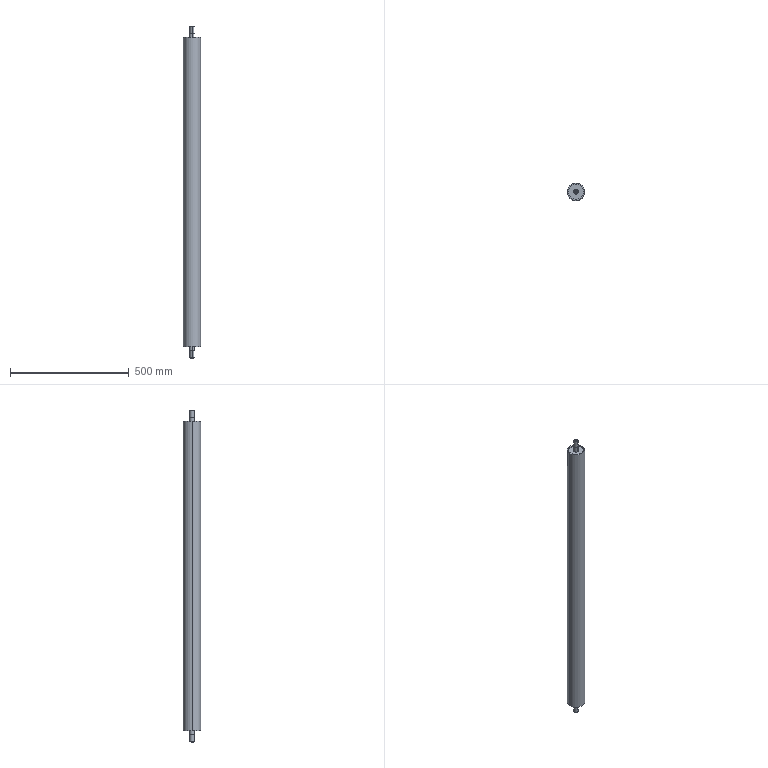Part | STEP file | Produce dryer-Driven part 2 | 1 solid | 44 faces | box 73 x 73 x 1397 mm | volume 1653987 mm3 | cylinder 22 | cone 12 | plane 10 | commonest cylinder face diameters 20 x6 64.52 x6 5 x4 17 x4 73 x2
STEP:
#1=CARTESIAN_POINT('',(2.5,0.,-683.5));
#2=VERTEX_POINT('',#1);
#3=CARTESIAN_POINT('',(-2.5,0.,-683.5));
#4=VERTEX_POINT('',#3);
#5=CARTESIAN_POINT('',(0.,0.,-683.5));
#6=DIRECTION('',(0.,0.,-1.));
#7=DIRECTION('',(-1.,0.,0.));
#8=AXIS2_PLACEMENT_3D('',#5,#6,#7);
#9=CIRCLE('',#8,2.5);
#10=EDGE_CURVE('',#2,#4,#9,.T.);
#11=ORIENTED_EDGE('',*,*,#10,.F.);
#12=CARTESIAN_POINT('',(2.5,0.,-698.5));
#13=VERTEX_POINT('',#12);
#14=CARTESIAN_POINT('',(2.5,0.,-698.5));
#15=DIRECTION('',(0.,0.,-1.));
#16=VECTOR('',#15,1000.);
#17=LINE('',#14,#16);
#18=EDGE_CURVE('',#2,#13,#17,.T.);
#19=ORIENTED_EDGE('',*,*,#18,.T.);
#20=CARTESIAN_POINT('',(-2.5,0.,-698.5));
#21=VERTEX_POINT('',#20);
#22=CARTESIAN_POINT('',(0.,0.,-698.5));
#23=DIRECTION('',(0.,0.,-1.));
#24=DIRECTION('',(-1.,0.,0.));
#25=AXIS2_PLACEMENT_3D('',#22,#23,#24);
#26=CIRCLE('',#25,2.5);
#27=EDGE_CURVE('',#13,#21,#26,.T.);
#28=ORIENTED_EDGE('',*,*,#27,.T.);
#29=CARTESIAN_POINT('',(-2.5,0.,-698.5));
#30=DIRECTION('',(0.,0.,-1.));
#31=VECTOR('',#30,1000.);
#32=LINE('',#29,#31);
#33=EDGE_CURVE('',#4,#21,#32,.T.);
#34=ORIENTED_EDGE('',*,*,#33,.F.);
#35=EDGE_LOOP('',(#11,#19,#28,#34));
#36=FACE_OUTER_BOUND('',#35,.T.);
#37=CARTESIAN_POINT('',(0.,0.,-698.5));
#38=DIRECTION('',(0.,0.,-1.));
#39=DIRECTION('',(-1.,0.,0.));
#40=AXIS2_PLACEMENT_3D('',#37,#38,#39);
#41=CYLINDRICAL_SURFACE('',#40,2.5);
#42=ADVANCED_FACE('',(#36),#41,.F.);
#43=CARTESIAN_POINT('',(0.,0.,-681.998));
#44=VERTEX_POINT('',#43);
#45=CARTESIAN_POINT('',(-2.5,0.,-683.5));
#46=DIRECTION('',(-0.8572,0.,-0.515));
#47=VECTOR('',#46,1000.);
#48=LINE('',#45,#47);
#49=EDGE_CURVE('',#44,#4,#48,.T.);
#50=ORIENTED_EDGE('',*,*,#49,.F.);
#51=CARTESIAN_POINT('',(2.5,0.,-683.5));
#52=DIRECTION('',(0.8572,0.,-0.515));
#53=VECTOR('',#52,1000.);
#54=LINE('',#51,#53);
#55=EDGE_CURVE('',#44,#2,#54,.T.);
#56=ORIENTED_EDGE('',*,*,#55,.T.);
#57=ORIENTED_EDGE('',*,*,#10,.T.);
#58=EDGE_LOOP('',(#50,#56,#57));
#59=FACE_OUTER_BOUND('',#58,.T.);
#60=CARTESIAN_POINT('',(0.,0.,-683.5));
#61=DIRECTION('',(0.,0.,-1.));
#62=DIRECTION('',(-1.,0.,0.));
#63=AXIS2_PLACEMENT_3D('',#60,#61,#62);
#64=CONICAL_SURFACE('',#63,2.5,1.03);
#65=ADVANCED_FACE('',(#59),#64,.F.);
#66=CARTESIAN_POINT('',(0.,-10.,-667.));
#67=VERTEX_POINT('',#66);
#68=CARTESIAN_POINT('',(0.,10.,-667.));
#69=VERTEX_POINT('',#68);
#70=CARTESIAN_POINT('',(0.,0.,-667.));
#71=DIRECTION('',(0.,0.,1.));
#72=DIRECTION('',(0.,-1.,0.));
#73=AXIS2_PLACEMENT_3D('',#70,#71,#72);
#74=CIRCLE('',#73,10.);
#75=EDGE_CURVE('',#67,#69,#74,.T.);
#76=ORIENTED_EDGE('',*,*,#75,.T.);
#77=CARTESIAN_POINT('',(0.,10.,-645.5));
#78=VERTEX_POINT('',#77);
#79=CARTESIAN_POINT('',(0.,10.,-698.5));
#80=DIRECTION('',(0.,0.,1.));
#81=VECTOR('',#80,1000.);
#82=LINE('',#79,#81);
#83=EDGE_CURVE('',#69,#78,#82,.T.);
#84=ORIENTED_EDGE('',*,*,#83,.T.);
#85=CARTESIAN_POINT('',(0.,-10.,-645.5));
#86=VERTEX_POINT('',#85);
#87=CARTESIAN_POINT('',(0.,0.,-645.5));
#88=DIRECTION('',(0.,0.,-1.));
#89=DIRECTION('',(-1.,0.,0.));
#90=AXIS2_PLACEMENT_3D('',#87,#88,#89);
#91=CIRCLE('',#90,10.);
#92=EDGE_CURVE('',#78,#86,#91,.T.);
#93=ORIENTED_EDGE('',*,*,#92,.T.);
#94=CARTESIAN_POINT('',(0.,-10.,-698.5));
#95=DIRECTION('',(0.,0.,1.));
#96=VECTOR('',#95,1000.);
#97=LINE('',#94,#96);
#98=EDGE_CURVE('',#67,#86,#97,.T.);
#99=ORIENTED_EDGE('',*,*,#98,.F.);
#100=EDGE_LOOP('',(#76,#84,#93,#99));
#101=FACE_OUTER_BOUND('',#100,.T.);
#102=CARTESIAN_POINT('',(0.,0.,-698.5));
#103=DIRECTION('',(0.,0.,1.));
#104=DIRECTION('',(0.,-1.,0.));
#105=AXIS2_PLACEMENT_3D('',#102,#103,#104);
#106=CYLINDRICAL_SURFACE('',#105,10.);
#107=ADVANCED_FACE('',(#101),#106,.T.);
#108=CARTESIAN_POINT('',(0.,9.5,-667.5));
#109=VERTEX_POINT('',#108);
#110=CARTESIAN_POINT('',(0.,-9.5,-667.5));
#111=VERTEX_POINT('',#110);
#112=CARTESIAN_POINT('',(0.,0.,-667.5));
#113=DIRECTION('',(0.,0.,-1.));
#114=DIRECTION('',(0.,-1.,0.));
#115=AXIS2_PLACEMENT_3D('',#112,#113,#114);
#116=CIRCLE('',#115,9.5);
#117=EDGE_CURVE('',#109,#111,#116,.T.);
#118=ORIENTED_EDGE('',*,*,#117,.F.);
#119=CARTESIAN_POINT('',(0.,10.,-667.));
#120=DIRECTION('',(0.,0.7071,0.7071));
#121=VECTOR('',#120,1000.);
#122=LINE('',#119,#121);
#123=EDGE_CURVE('',#109,#69,#122,.T.);
#124=ORIENTED_EDGE('',*,*,#123,.T.);
#125=ORIENTED_EDGE('',*,*,#75,.F.);
#126=CARTESIAN_POINT('',(0.,-10.,-667.));
#127=DIRECTION('',(0.,-0.7071,0.7071));
#128=VECTOR('',#127,1000.);
#129=LINE('',#126,#128);
#130=EDGE_CURVE('',#111,#67,#129,.T.);
#131=ORIENTED_EDGE('',*,*,#130,.F.);
#132=EDGE_LOOP('',(#118,#124,#125,#131));
#133=FACE_OUTER_BOUND('',#132,.T.);
#134=CARTESIAN_POINT('',(0.,0.,-667.));
#135=DIRECTION('',(0.,0.,1.));
#136=DIRECTION('',(0.,-1.,0.));
#137=AXIS2_PLACEMENT_3D('',#134,#135,#136);
#138=CONICAL_SURFACE('',#137,10.,0.7854);
#139=ADVANCED_FACE('',(#133),#138,.T.);
#140=CARTESIAN_POINT('',(0.,-8.5,-698.));
#141=VERTEX_POINT('',#140);
#142=CARTESIAN_POINT('',(0.,8.5,-698.));
#143=VERTEX_POINT('',#142);
#144=CARTESIAN_POINT('',(0.,0.,-698.));
#145=DIRECTION('',(0.,0.,1.));
#146=DIRECTION('',(0.,-1.,0.));
#147=AXIS2_PLACEMENT_3D('',#144,#145,#146);
#148=CIRCLE('',#147,8.5);
#149=EDGE_CURVE('',#141,#143,#148,.T.);
#150=ORIENTED_EDGE('',*,*,#149,.T.);
#151=CARTESIAN_POINT('',(0.,8.5,-667.5));
#152=VERTEX_POINT('',#151);
#153=CARTESIAN_POINT('',(0.,8.5,-698.5));
#154=DIRECTION('',(0.,0.,1.));
#155=VECTOR('',#154,1000.);
#156=LINE('',#153,#155);
#157=EDGE_CURVE('',#143,#152,#156,.T.);
#158=ORIENTED_EDGE('',*,*,#157,.T.);
#159=CARTESIAN_POINT('',(0.,-8.5,-667.5));
#160=VERTEX_POINT('',#159);
#161=CARTESIAN_POINT('',(0.,0.,-667.5));
#162=DIRECTION('',(0.,0.,1.));
#163=DIRECTION('',(0.,-1.,0.));
#164=AXIS2_PLACEMENT_3D('',#161,#162,#163);
#165=CIRCLE('',#164,8.5);
#166=EDGE_CURVE('',#160,#152,#165,.T.);
#167=ORIENTED_EDGE('',*,*,#166,.F.);
#168=CARTESIAN_POINT('',(0.,-8.5,-698.5));
#169=DIRECTION('',(0.,0.,1.));
#170=VECTOR('',#169,1000.);
#171=LINE('',#168,#170);
#172=EDGE_CURVE('',#141,#160,#171,.T.);
#173=ORIENTED_EDGE('',*,*,#172,.F.);
#174=EDGE_LOOP('',(#150,#158,#167,#173));
#175=FACE_OUTER_BOUND('',#174,.T.);
#176=CARTESIAN_POINT('',(0.,0.,-698.5));
#177=DIRECTION('',(0.,0.,1.));
#178=DIRECTION('',(0.,-1.,0.));
#179=AXIS2_PLACEMENT_3D('',#176,#177,#178);
#180=CYLINDRICAL_SURFACE('',#179,8.5);
#181=ADVANCED_FACE('',(#175),#180,.T.);
#182=CARTESIAN_POINT('',(0.,8.,-698.5));
#183=VERTEX_POINT('',#182);
#184=CARTESIAN_POINT('',(0.,-8.,-698.5));
#185=VERTEX_POINT('',#184);
#186=CARTESIAN_POINT('',(0.,0.,-698.5));
#187=DIRECTION('',(0.,0.,-1.));
#188=DIRECTION('',(0.,-1.,0.));
#189=AXIS2_PLACEMENT_3D('',#186,#187,#188);
#190=CIRCLE('',#189,8.);
#191=EDGE_CURVE('',#183,#185,#190,.T.);
#192=ORIENTED_EDGE('',*,*,#191,.F.);
#193=CARTESIAN_POINT('',(0.,8.5,-698.));
#194=DIRECTION('',(0.,0.7071,0.7071));
#195=VECTOR('',#194,1000.);
#196=LINE('',#193,#195);
#197=EDGE_CURVE('',#183,#143,#196,.T.);
#198=ORIENTED_EDGE('',*,*,#197,.T.);
#199=ORIENTED_EDGE('',*,*,#149,.F.);
#200=CARTESIAN_POINT('',(0.,-8.5,-698.));
#201=DIRECTION('',(0.,-0.7071,0.7071));
#202=VECTOR('',#201,1000.);
#203=LINE('',#200,#202);
#204=EDGE_CURVE('',#185,#141,#203,.T.);
#205=ORIENTED_EDGE('',*,*,#204,.F.);
#206=EDGE_LOOP('',(#192,#198,#199,#205));
#207=FACE_OUTER_BOUND('',#206,.T.);
#208=CARTESIAN_POINT('',(0.,0.,-698.));
#209=DIRECTION('',(0.,0.,1.));
#210=DIRECTION('',(0.,-1.,0.));
#211=AXIS2_PLACEMENT_3D('',#208,#209,#210);
#212=CONICAL_SURFACE('',#211,8.5,0.7854);
#213=ADVANCED_FACE('',(#207),#212,.T.);
#214=CARTESIAN_POINT('',(-2.5,0.,683.5));
#215=VERTEX_POINT('',#214);
#216=CARTESIAN_POINT('',(2.5,0.,683.5));
#217=VERTEX_POINT('',#216);
#218=CARTESIAN_POINT('',(0.,0.,683.5));
#219=DIRECTION('',(0.,0.,1.));
#220=DIRECTION('',(1.,0.,0.));
#221=AXIS2_PLACEMENT_3D('',#218,#219,#220);
#222=CIRCLE('',#221,2.5);
#223=EDGE_CURVE('',#215,#217,#222,.T.);
#224=ORIENTED_EDGE('',*,*,#223,.F.);
#225=CARTESIAN_POINT('',(-2.5,0.,698.5));
#226=VERTEX_POINT('',#225);
#227=CARTESIAN_POINT('',(-2.5,0.,698.5));
#228=DIRECTION('',(0.,0.,1.));
#229=VECTOR('',#228,1000.);
#230=LINE('',#227,#229);
#231=EDGE_CURVE('',#215,#226,#230,.T.);
#232=ORIENTED_EDGE('',*,*,#231,.T.);
#233=CARTESIAN_POINT('',(2.5,0.,698.5));
#234=VERTEX_POINT('',#233);
#235=CARTESIAN_POINT('',(0.,0.,698.5));
#236=DIRECTION('',(0.,0.,1.));
#237=DIRECTION('',(1.,0.,0.));
#238=AXIS2_PLACEMENT_3D('',#235,#236,#237);
#239=CIRCLE('',#238,2.5);
#240=EDGE_CURVE('',#226,#234,#239,.T.);
#241=ORIENTED_EDGE('',*,*,#240,.T.);
#242=CARTESIAN_POINT('',(2.5,0.,698.5));
#243=DIRECTION('',(0.,0.,1.));
#244=VECTOR('',#243,1000.);
#245=LINE('',#242,#244);
#246=EDGE_CURVE('',#217,#234,#245,.T.);
#247=ORIENTED_EDGE('',*,*,#246,.F.);
#248=EDGE_LOOP('',(#224,#232,#241,#247));
#249=FACE_OUTER_BOUND('',#248,.T.);
#250=CARTESIAN_POINT('',(0.,0.,698.5));
#251=DIRECTION('',(0.,0.,1.));
#252=DIRECTION('',(1.,0.,0.));
#253=AXIS2_PLACEMENT_3D('',#250,#251,#252);
#254=CYLINDRICAL_SURFACE('',#253,2.5);
#255=ADVANCED_FACE('',(#249),#254,.F.);
#256=CARTESIAN_POINT('',(0.,0.,681.998));
#257=VERTEX_POINT('',#256);
#258=CARTESIAN_POINT('',(2.5,0.,683.5));
#259=DIRECTION('',(0.8572,0.,0.515));
#260=VECTOR('',#259,1000.);
#261=LINE('',#258,#260);
#262=EDGE_CURVE('',#257,#217,#261,.T.);
#263=ORIENTED_EDGE('',*,*,#262,.F.);
#264=CARTESIAN_POINT('',(-2.5,0.,683.5));
#265=DIRECTION('',(-0.8572,0.,0.515));
#266=VECTOR('',#265,1000.);
#267=LINE('',#264,#266);
#268=EDGE_CURVE('',#257,#215,#267,.T.);
#269=ORIENTED_EDGE('',*,*,#268,.T.);
#270=ORIENTED_EDGE('',*,*,#223,.T.);
#271=EDGE_LOOP('',(#263,#269,#270));
#272=FACE_OUTER_BOUND('',#271,.T.);
#273=CARTESIAN_POINT('',(0.,0.,683.5));
#274=DIRECTION('',(0.,0.,1.));
#275=DIRECTION('',(1.,0.,0.));
#276=AXIS2_PLACEMENT_3D('',#273,#274,#275);
#277=CONICAL_SURFACE('',#276,2.5,1.03);
#278=ADVANCED_FACE('',(#272),#277,.F.);
#279=CARTESIAN_POINT('',(0.,-9.5,667.5));
#280=VERTEX_POINT('',#279);
#281=CARTESIAN_POINT('',(0.,9.5,667.5));
#282=VERTEX_POINT('',#281);
#283=CARTESIAN_POINT('',(0.,0.,667.5));
#284=DIRECTION('',(0.,0.,1.));
#285=DIRECTION('',(0.,1.,0.));
#286=AXIS2_PLACEMENT_3D('',#283,#284,#285);
#287=CIRCLE('',#286,9.5);
#288=EDGE_CURVE('',#280,#282,#287,.T.);
#289=ORIENTED_EDGE('',*,*,#288,.F.);
#290=CARTESIAN_POINT('',(0.,-10.,667.));
#291=VERTEX_POINT('',#290);
#292=CARTESIAN_POINT('',(0.,-9.5,667.5));
#293=DIRECTION('',(0.,-0.7071,-0.7071));
#294=VECTOR('',#293,1000.);
#295=LINE('',#292,#294);
#296=EDGE_CURVE('',#280,#291,#295,.T.);
#297=ORIENTED_EDGE('',*,*,#296,.T.);
#298=CARTESIAN_POINT('',(0.,10.,667.));
#299=VERTEX_POINT('',#298);
#300=CARTESIAN_POINT('',(0.,0.,667.));
#301=DIRECTION('',(0.,0.,-1.));
#302=DIRECTION('',(0.,1.,0.));
#303=AXIS2_PLACEMENT_3D('',#300,#301,#302);
#304=CIRCLE('',#303,10.);
#305=EDGE_CURVE('',#299,#291,#304,.T.);
#306=ORIENTED_EDGE('',*,*,#305,.F.);
#307=CARTESIAN_POINT('',(0.,9.5,667.5));
#308=DIRECTION('',(0.,0.7071,-0.7071));
#309=VECTOR('',#308,1000.);
#310=LINE('',#307,#309);
#311=EDGE_CURVE('',#282,#299,#310,.T.);
#312=ORIENTED_EDGE('',*,*,#311,.F.);
#313=EDGE_LOOP('',(#289,#297,#306,#312));
#314=FACE_OUTER_BOUND('',#313,.T.);
#315=CARTESIAN_POINT('',(0.,0.,667.5));
#316=DIRECTION('',(0.,0.,-1.));
#317=DIRECTION('',(0.,1.,0.));
#318=AXIS2_PLACEMENT_3D('',#315,#316,#317);
#319=CONICAL_SURFACE('',#318,9.5,0.7854);
#320=ADVANCED_FACE('',(#314),#319,.T.);
#321=CARTESIAN_POINT('',(0.,-8.,698.5));
#322=VERTEX_POINT('',#321);
#323=CARTESIAN_POINT('',(0.,8.,698.5));
#324=VERTEX_POINT('',#323);
#325=CARTESIAN_POINT('',(0.,0.,698.5));
#326=DIRECTION('',(0.,0.,1.));
#327=DIRECTION('',(0.,1.,0.));
#328=AXIS2_PLACEMENT_3D('',#325,#326,#327);
#329=CIRCLE('',#328,8.);
#330=EDGE_CURVE('',#322,#324,#329,.T.);
#331=ORIENTED_EDGE('',*,*,#330,.F.);
#332=CARTESIAN_POINT('',(0.,-8.5,698.));
#333=VERTEX_POINT('',#332);
#334=CARTESIAN_POINT('',(0.,-8.,698.5));
#335=DIRECTION('',(0.,-0.7071,-0.7071));
#336=VECTOR('',#335,1000.);
#337=LINE('',#334,#336);
#338=EDGE_CURVE('',#322,#333,#337,.T.);
#339=ORIENTED_EDGE('',*,*,#338,.T.);
#340=CARTESIAN_POINT('',(0.,8.5,698.));
#341=VERTEX_POINT('',#340);
#342=CARTESIAN_POINT('',(0.,0.,698.));
#343=DIRECTION('',(0.,0.,-1.));
#344=DIRECTION('',(0.,1.,0.));
#345=AXIS2_PLACEMENT_3D('',#342,#343,#344);
#346=CIRCLE('',#345,8.5);
#347=EDGE_CURVE('',#341,#333,#346,.T.);
#348=ORIENTED_EDGE('',*,*,#347,.F.);
#349=CARTESIAN_POINT('',(0.,8.,698.5));
#350=DIRECTION('',(0.,0.7071,-0.7071));
#351=VECTOR('',#350,1000.);
#352=LINE('',#349,#351);
#353=EDGE_CURVE('',#324,#341,#352,.T.);
#354=ORIENTED_EDGE('',*,*,#353,.F.);
#355=EDGE_LOOP('',(#331,#339,#348,#354));
#356=FACE_OUTER_BOUND('',#355,.T.);
#357=CARTESIAN_POINT('',(0.,0.,698.5));
#358=DIRECTION('',(0.,0.,-1.));
#359=DIRECTION('',(0.,1.,0.));
#360=AXIS2_PLACEMENT_3D('',#357,#358,#359);
#361=CONICAL_SURFACE('',#360,8.,0.7854);
#362=ADVANCED_FACE('',(#356),#361,.T.);
#363=CARTESIAN_POINT('',(0.,10.,645.5));
#364=VERTEX_POINT('',#363);
#365=CARTESIAN_POINT('',(0.,-10.,645.5));
#366=VERTEX_POINT('',#365);
#367=CARTESIAN_POINT('',(0.,0.,645.5));
#368=DIRECTION('',(0.,0.,-1.));
#369=DIRECTION('',(1.,0.,0.));
#370=AXIS2_PLACEMENT_3D('',#367,#368,#369);
#371=CIRCLE('',#370,10.);
#372=EDGE_CURVE('',#364,#366,#371,.T.);
#373=ORIENTED_EDGE('',*,*,#372,.F.);
#374=CARTESIAN_POINT('',(0.,10.,-698.5));
#375=DIRECTION('',(0.,0.,1.));
#376=VECTOR('',#375,1000.);
#377=LINE('',#374,#376);
#378=EDGE_CURVE('',#364,#299,#377,.T.);
#379=ORIENTED_EDGE('',*,*,#378,.T.);
#380=ORIENTED_EDGE('',*,*,#305,.T.);
#381=CARTESIAN_POINT('',(0.,-10.,-698.5));
#382=DIRECTION('',(0.,0.,1.));
#383=VECTOR('',#382,1000.);
#384=LINE('',#381,#383);
#385=EDGE_CURVE('',#366,#291,#384,.T.);
#386=ORIENTED_EDGE('',*,*,#385,.F.);
#387=EDGE_LOOP('',(#373,#379,#380,#386));
#388=FACE_OUTER_BOUND('',#387,.T.);
#389=CARTESIAN_POINT('',(0.,0.,-698.5));
#390=DIRECTION('',(0.,0.,1.));
#391=DIRECTION('',(0.,-1.,0.));
#392=AXIS2_PLACEMENT_3D('',#389,#390,#391);
#393=CYLINDRICAL_SURFACE('',#392,10.);
#394=ADVANCED_FACE('',(#388),#393,.T.);
#395=CARTESIAN_POINT('',(0.,-8.5,667.5));
#396=VERTEX_POINT('',#395);
#397=CARTESIAN_POINT('',(0.,8.5,667.5));
#398=VERTEX_POINT('',#397);
#399=CARTESIAN_POINT('',(0.,0.,667.5));
#400=DIRECTION('',(0.,0.,1.));
#401=DIRECTION('',(0.,-1.,0.));
#402=AXIS2_PLACEMENT_3D('',#399,#400,#401);
#403=CIRCLE('',#402,8.5);
#404=EDGE_CURVE('',#396,#398,#403,.T.);
#405=ORIENTED_EDGE('',*,*,#404,.T.);
#406=CARTESIAN_POINT('',(0.,8.5,-698.5));
#407=DIRECTION('',(0.,0.,1.));
#408=VECTOR('',#407,1000.);
#409=LINE('',#406,#408);
#410=EDGE_CURVE('',#398,#341,#409,.T.);
#411=ORIENTED_EDGE('',*,*,#410,.T.);
#412=ORIENTED_EDGE('',*,*,#347,.T.);
#413=CARTESIAN_POINT('',(0.,-8.5,-698.5));
#414=DIRECTION('',(0.,0.,1.));
#415=VECTOR('',#414,1000.);
#416=LINE('',#413,#415);
#417=EDGE_CURVE('',#396,#333,#416,.T.);
#418=ORIENTED_EDGE('',*,*,#417,.F.);
#419=EDGE_LOOP('',(#405,#411,#412,#418));
#420=FACE_OUTER_BOUND('',#419,.T.);
#421=CARTESIAN_POINT('',(0.,0.,-698.5));
#422=DIRECTION('',(0.,0.,1.));
#423=DIRECTION('',(0.,-1.,0.));
#424=AXIS2_PLACEMENT_3D('',#421,#422,#423);
#425=CYLINDRICAL_SURFACE('',#424,8.5);
#426=ADVANCED_FACE('',(#420),#425,.T.);
#427=CARTESIAN_POINT('',(-32.26,0.,650.5));
#428=VERTEX_POINT('',#427);
#429=CARTESIAN_POINT('',(32.26,0.,650.5));
#430=VERTEX_POINT('',#429);
#431=CARTESIAN_POINT('',(0.,0.,650.5));
#432=DIRECTION('',(0.,0.,1.));
#433=DIRECTION('',(1.,0.,0.));
#434=AXIS2_PLACEMENT_3D('',#431,#432,#433);
#435=CIRCLE('',#434,32.26);
#436=EDGE_CURVE('',#428,#430,#435,.T.);
#437=ORIENTED_EDGE('',*,*,#436,.T.);
#438=CARTESIAN_POINT('',(32.26,0.,645.5));
#439=VERTEX_POINT('',#438);
#440=CARTESIAN_POINT('',(32.26,0.,650.5));
#441=DIRECTION('',(0.,0.,-1.));
#442=VECTOR('',#441,1000.);
#443=LINE('',#440,#442);
#444=EDGE_CURVE('',#430,#439,#443,.T.);
#445=ORIENTED_EDGE('',*,*,#444,.T.);
#446=CARTESIAN_POINT('',(-32.26,0.,645.5));
#447=VERTEX_POINT('',#446);
#448=CARTESIAN_POINT('',(0.,0.,645.5));
#449=DIRECTION('',(0.,0.,1.));
#450=DIRECTION('',(1.,0.,0.));
#451=AXIS2_PLACEMENT_3D('',#448,#449,#450);
#452=CIRCLE('',#451,32.26);
#453=EDGE_CURVE('',#447,#439,#452,.T.);
#454=ORIENTED_EDGE('',*,*,#453,.F.);
#455=CARTESIAN_POINT('',(-32.26,0.,650.5));
#456=DIRECTION('',(0.,0.,-1.));
#457=VECTOR('',#456,1000.);
#458=LINE('',#455,#457);
#459=EDGE_CURVE('',#428,#447,#458,.T.);
#460=ORIENTED_EDGE('',*,*,#459,.F.);
#461=EDGE_LOOP('',(#437,#445,#454,#460));
#462=FACE_OUTER_BOUND('',#461,.T.);
#463=CARTESIAN_POINT('',(0.,0.,650.5));
#464=DIRECTION('',(0.,0.,-1.));
#465=DIRECTION('',(-1.,0.,0.));
#466=AXIS2_PLACEMENT_3D('',#463,#464,#465);
#467=CYLINDRICAL_SURFACE('',#466,32.26);
#468=ADVANCED_FACE('',(#462),#467,.F.);
#469=CARTESIAN_POINT('',(36.5,0.,650.5));
#470=VERTEX_POINT('',#469);
#471=CARTESIAN_POINT('',(-36.5,0.,650.5));
#472=VERTEX_POINT('',#471);
#473=CARTESIAN_POINT('',(0.,0.,650.5));
#474=DIRECTION('',(0.,0.,1.));
#475=DIRECTION('',(1.,0.,0.));
#476=AXIS2_PLACEMENT_3D('',#473,#474,#475);
#477=CIRCLE('',#476,36.5);
#478=EDGE_CURVE('',#470,#472,#477,.T.);
#479=ORIENTED_EDGE('',*,*,#478,.F.);
#480=CARTESIAN_POINT('',(36.5,0.,-650.5));
#481=VERTEX_POINT('',#480);
#482=CARTESIAN_POINT('',(36.5,0.,650.5));
#483=DIRECTION('',(0.,0.,-1.));
#484=VECTOR('',#483,1000.);
#485=LINE('',#482,#484);
#486=EDGE_CURVE('',#470,#481,#485,.T.);
#487=ORIENTED_EDGE('',*,*,#486,.T.);
#488=CARTESIAN_POINT('',(-36.5,0.,-650.5));
#489=VERTEX_POINT('',#488);
#490=CARTESIAN_POINT('',(0.,0.,-650.5));
#491=DIRECTION('',(0.,0.,1.));
#492=DIRECTION('',(1.,0.,0.));
#493=AXIS2_PLACEMENT_3D('',#490,#491,#492);
#494=CIRCLE('',#493,36.5);
#495=EDGE_CURVE('',#481,#489,#494,.T.);
#496=ORIENTED_EDGE('',*,*,#495,.T.);
#497=CARTESIAN_POINT('',(-36.5,0.,650.5));
#498=DIRECTION('',(0.,0.,-1.));
#499=VECTOR('',#498,1000.);
#500=LINE('',#497,#499);
#501=EDGE_CURVE('',#472,#489,#500,.T.);
#502=ORIENTED_EDGE('',*,*,#501,.F.);
#503=EDGE_LOOP('',(#479,#487,#496,#502));
#504=FACE_OUTER_BOUND('',#503,.T.);
#505=CARTESIAN_POINT('',(0.,0.,650.5));
#506=DIRECTION('',(0.,0.,-1.));
#507=DIRECTION('',(-1.,0.,0.));
#508=AXIS2_PLACEMENT_3D('',#505,#506,#507);
#509=CYLINDRICAL_SURFACE('',#508,36.5);
#510=ADVANCED_FACE('',(#504),#509,.T.);
#511=CARTESIAN_POINT('',(32.26,0.,-645.5));
#512=VERTEX_POINT('',#511);
#513=CARTESIAN_POINT('',(-32.26,0.,-645.5));
#514=VERTEX_POINT('',#513);
#515=CARTESIAN_POINT('',(0.,0.,-645.5));
#516=DIRECTION('',(0.,0.,-1.));
#517=DIRECTION('',(-1.,0.,0.));
#518=AXIS2_PLACEMENT_3D('',#515,#516,#517);
#519=CIRCLE('',#518,32.26);
#520=EDGE_CURVE('',#512,#514,#519,.T.);
#521=ORIENTED_EDGE('',*,*,#520,.F.);
#522=CARTESIAN_POINT('',(32.26,0.,-650.5));
#523=VERTEX_POINT('',#522);
#524=CARTESIAN_POINT('',(32.26,0.,650.5));
#525=DIRECTION('',(0.,0.,-1.));
#526=VECTOR('',#525,1000.);
#527=LINE('',#524,#526);
#528=EDGE_CURVE('',#512,#523,#527,.T.);
#529=ORIENTED_EDGE('',*,*,#528,.T.);
#530=CARTESIAN_POINT('',(-32.26,0.,-650.5));
#531=VERTEX_POINT('',#530);
#532=CARTESIAN_POINT('',(0.,0.,-650.5));
#533=DIRECTION('',(0.,0.,1.));
#534=DIRECTION('',(1.,0.,0.));
#535=AXIS2_PLACEMENT_3D('',#532,#533,#534);
#536=CIRCLE('',#535,32.26);
#537=EDGE_CURVE('',#531,#523,#536,.T.);
#538=ORIENTED_EDGE('',*,*,#537,.F.);
#539=CARTESIAN_POINT('',(-32.26,0.,650.5));
#540=DIRECTION('',(0.,0.,-1.));
#541=VECTOR('',#540,1000.);
#542=LINE('',#539,#541);
#543=EDGE_CURVE('',#514,#531,#542,.T.);
#544=ORIENTED_EDGE('',*,*,#543,.F.);
#545=EDGE_LOOP('',(#521,#529,#538,#544));
#546=FACE_OUTER_BOUND('',#545,.T.);
#547=CARTESIAN_POINT('',(0.,0.,650.5));
#548=DIRECTION('',(0.,0.,-1.));
#549=DIRECTION('',(-1.,0.,0.));
#550=AXIS2_PLACEMENT_3D('',#547,#548,#549);
#551=CYLINDRICAL_SURFACE('',#550,32.26);
#552=ADVANCED_FACE('',(#546),#551,.F.);
#553=ORIENTED_EDGE('',*,*,#528,.F.);
#554=CARTESIAN_POINT('',(0.,0.,-645.5));
#555=DIRECTION('',(0.,0.,-1.));
#556=DIRECTION('',(-1.,0.,0.));
#557=AXIS2_PLACEMENT_3D('',#554,#555,#556);
#558=CIRCLE('',#557,32.26);
#559=EDGE_CURVE('',#514,#512,#558,.T.);
#560=ORIENTED_EDGE('',*,*,#559,.F.);
#561=ORIENTED_EDGE('',*,*,#543,.T.);
#562=CARTESIAN_POINT('',(0.,0.,-650.5));
#563=DIRECTION('',(0.,0.,1.));
#564=DIRECTION('',(1.,0.,0.));
#565=AXIS2_PLACEMENT_3D('',#562,#563,#564);
#566=CIRCLE('',#565,32.26);
#567=EDGE_CURVE('',#523,#531,#566,.T.);
#568=ORIENTED_EDGE('',*,*,#567,.F.);
#569=EDGE_LOOP('',(#553,#560,#561,#568));
#570=FACE_OUTER_BOUND('',#569,.T.);
#571=CARTESIAN_POINT('',(0.,0.,650.5));
#572=DIRECTION('',(0.,0.,-1.));
#573=DIRECTION('',(-1.,0.,0.));
#574=AXIS2_PLACEMENT_3D('',#571,#572,#573);
#575=CYLINDRICAL_SURFACE('',#574,32.26);
#576=ADVANCED_FACE('',(#570),#575,.F.);
#577=CARTESIAN_POINT('',(0.,0.,650.5));
#578=DIRECTION('',(0.,0.,1.));
#579=DIRECTION('',(1.,0.,0.));
#580=AXIS2_PLACEMENT_3D('',#577,#578,#579);
#581=CIRCLE('',#580,36.5);
#582=EDGE_CURVE('',#472,#470,#581,.T.);
#583=ORIENTED_EDGE('',*,*,#582,.T.);
#584=ORIENTED_EDGE('',*,*,#478,.T.);
#585=EDGE_LOOP('',(#583,#584));
#586=FACE_OUTER_BOUND('',#585,.T.);
#587=ORIENTED_EDGE('',*,*,#436,.F.);
#588=CARTESIAN_POINT('',(0.,0.,650.5));
#589=DIRECTION('',(0.,0.,1.));
#590=DIRECTION('',(1.,0.,0.));
#591=AXIS2_PLACEMENT_3D('',#588,#589,#590);
#592=CIRCLE('',#591,32.26);
#593=EDGE_CURVE('',#430,#428,#592,.T.);
#594=ORIENTED_EDGE('',*,*,#593,.F.);
#595=EDGE_LOOP('',(#587,#594));
#596=FACE_BOUND('',#595,.T.);
#597=CARTESIAN_POINT('',(0.,0.,650.5));
#598=DIRECTION('',(0.,0.,1.));
#599=DIRECTION('',(1.,0.,0.));
#600=AXIS2_PLACEMENT_3D('',#597,#598,#599);
#601=PLANE('',#600);
#602=ADVANCED_FACE('',(#586,#596),#601,.T.);
#603=CARTESIAN_POINT('',(0.,0.,-650.5));
#604=DIRECTION('',(0.,0.,1.));
#605=DIRECTION('',(1.,0.,0.));
#606=AXIS2_PLACEMENT_3D('',#603,#604,#605);
#607=CIRCLE('',#606,36.5);
#608=EDGE_CURVE('',#489,#481,#607,.T.);
#609=ORIENTED_EDGE('',*,*,#608,.F.);
#610=ORIENTED_EDGE('',*,*,#495,.F.);
#611=EDGE_LOOP('',(#609,#610));
#612=FACE_OUTER_BOUND('',#611,.T.);
#613=ORIENTED_EDGE('',*,*,#537,.T.);
#614=ORIENTED_EDGE('',*,*,#567,.T.);
#615=EDGE_LOOP('',(#613,#614));
#616=FACE_BOUND('',#615,.T.);
#617=CARTESIAN_POINT('',(0.,0.,-650.5));
#618=DIRECTION('',(0.,0.,1.));
#619=DIRECTION('',(1.,0.,0.));
#620=AXIS2_PLACEMENT_3D('',#617,#618,#619);
#621=PLANE('',#620);
#622=ADVANCED_FACE('',(#612,#616),#621,.F.);
#623=ORIENTED_EDGE('',*,*,#486,.F.);
#624=ORIENTED_EDGE('',*,*,#582,.F.);
#625=ORIENTED_EDGE('',*,*,#501,.T.);
#626=ORIENTED_EDGE('',*,*,#608,.T.);
#627=EDGE_LOOP('',(#623,#624,#625,#626));
#628=FACE_OUTER_BOUND('',#627,.T.);
#629=CARTESIAN_POINT('',(0.,0.,650.5));
#630=DIRECTION('',(0.,0.,-1.));
#631=DIRECTION('',(-1.,0.,0.));
#632=AXIS2_PLACEMENT_3D('',#629,#630,#631);
#633=CYLINDRICAL_SURFACE('',#632,36.5);
#634=ADVANCED_FACE('',(#628),#633,.T.);
#635=ORIENTED_EDGE('',*,*,#444,.F.);
#636=ORIENTED_EDGE('',*,*,#593,.T.);
#637=ORIENTED_EDGE('',*,*,#459,.T.);
#638=CARTESIAN_POINT('',(0.,0.,645.5));
#639=DIRECTION('',(0.,0.,1.));
#640=DIRECTION('',(1.,0.,0.));
#641=AXIS2_PLACEMENT_3D('',#638,#639,#640);
#642=CIRCLE('',#641,32.26);
#643=EDGE_CURVE('',#439,#447,#642,.T.);
#644=ORIENTED_EDGE('',*,*,#643,.F.);
#645=EDGE_LOOP('',(#635,#636,#637,#644));
#646=FACE_OUTER_BOUND('',#645,.T.);
#647=CARTESIAN_POINT('',(0.,0.,650.5));
#648=DIRECTION('',(0.,0.,-1.));
#649=DIRECTION('',(-1.,0.,0.));
#650=AXIS2_PLACEMENT_3D('',#647,#648,#649);
#651=CYLINDRICAL_SURFACE('',#650,32.26);
#652=ADVANCED_FACE('',(#646),#651,.F.);
#653=CARTESIAN_POINT('',(0.,0.,645.5));
#654=DIRECTION('',(0.,0.,-1.));
#655=DIRECTION('',(1.,0.,0.));
#656=AXIS2_PLACEMENT_3D('',#653,#654,#655);
#657=CIRCLE('',#656,10.);
#658=EDGE_CURVE('',#366,#364,#657,.T.);
#659=ORIENTED_EDGE('',*,*,#658,.T.);
#660=ORIENTED_EDGE('',*,*,#372,.T.);
#661=EDGE_LOOP('',(#659,#660));
#662=FACE_BOUND('',#661,.T.);
#663=ORIENTED_EDGE('',*,*,#453,.T.);
#664=ORIENTED_EDGE('',*,*,#643,.T.);
#665=EDGE_LOOP('',(#663,#664));
#666=FACE_OUTER_BOUND('',#665,.T.);
#667=CARTESIAN_POINT('',(0.,0.,645.5));
#668=DIRECTION('',(0.,0.,1.));
#669=DIRECTION('',(1.,0.,0.));
#670=AXIS2_PLACEMENT_3D('',#667,#668,#669);
#671=PLANE('',#670);
#672=ADVANCED_FACE('',(#662,#666),#671,.T.);
#673=CARTESIAN_POINT('',(0.,0.,698.5));
#674=DIRECTION('',(0.,0.,1.));
#675=DIRECTION('',(1.,0.,0.));
#676=AXIS2_PLACEMENT_3D('',#673,#674,#675);
#677=CIRCLE('',#676,2.5);
#678=EDGE_CURVE('',#234,#226,#677,.T.);
#679=ORIENTED_EDGE('',*,*,#678,.F.);
#680=ORIENTED_EDGE('',*,*,#240,.F.);
#681=EDGE_LOOP('',(#679,#680));
#682=FACE_BOUND('',#681,.T.);
#683=CARTESIAN_POINT('',(0.,0.,698.5));
#684=DIRECTION('',(0.,0.,1.));
#685=DIRECTION('',(0.,1.,0.));
#686=AXIS2_PLACEMENT_3D('',#683,#684,#685);
#687=CIRCLE('',#686,8.);
#688=EDGE_CURVE('',#324,#322,#687,.T.);
#689=ORIENTED_EDGE('',*,*,#688,.T.);
#690=ORIENTED_EDGE('',*,*,#330,.T.);
#691=EDGE_LOOP('',(#689,#690));
#692=FACE_OUTER_BOUND('',#691,.T.);
#693=CARTESIAN_POINT('',(0.,0.,698.5));
#694=DIRECTION('',(0.,0.,-1.));
#695=DIRECTION('',(0.,1.,0.));
#696=AXIS2_PLACEMENT_3D('',#693,#694,#695);
#697=PLANE('',#696);
#698=ADVANCED_FACE('',(#682,#692),#697,.F.);
#699=ORIENTED_EDGE('',*,*,#410,.F.);
#700=CARTESIAN_POINT('',(0.,0.,667.5));
#701=DIRECTION('',(0.,0.,1.));
#702=DIRECTION('',(0.,-1.,0.));
#703=AXIS2_PLACEMENT_3D('',#700,#701,#702);
#704=CIRCLE('',#703,8.5);
#705=EDGE_CURVE('',#398,#396,#704,.T.);
#706=ORIENTED_EDGE('',*,*,#705,.T.);
#707=ORIENTED_EDGE('',*,*,#417,.T.);
#708=CARTESIAN_POINT('',(0.,0.,698.));
#709=DIRECTION('',(0.,0.,-1.));
#710=DIRECTION('',(0.,1.,0.));
#711=AXIS2_PLACEMENT_3D('',#708,#709,#710);
#712=CIRCLE('',#711,8.5);
#713=EDGE_CURVE('',#333,#341,#712,.T.);
#714=ORIENTED_EDGE('',*,*,#713,.T.);
#715=EDGE_LOOP('',(#699,#706,#707,#714));
#716=FACE_OUTER_BOUND('',#715,.T.);
#717=CARTESIAN_POINT('',(0.,0.,-698.5));
#718=DIRECTION('',(0.,0.,1.));
#719=DIRECTION('',(0.,-1.,0.));
#720=AXIS2_PLACEMENT_3D('',#717,#718,#719);
#721=CYLINDRICAL_SURFACE('',#720,8.5);
#722=ADVANCED_FACE('',(#716),#721,.T.);
#723=CARTESIAN_POINT('',(0.,0.,667.5));
#724=DIRECTION('',(0.,0.,1.));
#725=DIRECTION('',(0.,1.,0.));
#726=AXIS2_PLACEMENT_3D('',#723,#724,#725);
#727=CIRCLE('',#726,9.5);
#728=EDGE_CURVE('',#282,#280,#727,.T.);
#729=ORIENTED_EDGE('',*,*,#728,.T.);
#730=ORIENTED_EDGE('',*,*,#288,.T.);
#731=EDGE_LOOP('',(#729,#730));
#732=FACE_OUTER_BOUND('',#731,.T.);
#733=ORIENTED_EDGE('',*,*,#404,.F.);
#734=ORIENTED_EDGE('',*,*,#705,.F.);
#735=EDGE_LOOP('',(#733,#734));
#736=FACE_BOUND('',#735,.T.);
#737=CARTESIAN_POINT('',(0.,8.5,667.5));
#738=DIRECTION('',(0.,0.,-1.));
#739=DIRECTION('',(0.,1.,0.));
#740=AXIS2_PLACEMENT_3D('',#737,#738,#739);
#741=PLANE('',#740);
#742=ADVANCED_FACE('',(#732,#736),#741,.F.);
#743=ORIENTED_EDGE('',*,*,#378,.F.);
#744=ORIENTED_EDGE('',*,*,#658,.F.);
#745=ORIENTED_EDGE('',*,*,#385,.T.);
#746=CARTESIAN_POINT('',(0.,0.,667.));
#747=DIRECTION('',(0.,0.,-1.));
#748=DIRECTION('',(0.,1.,0.));
#749=AXIS2_PLACEMENT_3D('',#746,#747,#748);
#750=CIRCLE('',#749,10.);
#751=EDGE_CURVE('',#291,#299,#750,.T.);
#752=ORIENTED_EDGE('',*,*,#751,.T.);
#753=EDGE_LOOP('',(#743,#744,#745,#752));
#754=FACE_OUTER_BOUND('',#753,.T.);
#755=CARTESIAN_POINT('',(0.,0.,-698.5));
#756=DIRECTION('',(0.,0.,1.));
#757=DIRECTION('',(0.,-1.,0.));
#758=AXIS2_PLACEMENT_3D('',#755,#756,#757);
#759=CYLINDRICAL_SURFACE('',#758,10.);
#760=ADVANCED_FACE('',(#754),#759,.T.);
#761=ORIENTED_EDGE('',*,*,#338,.F.);
#762=ORIENTED_EDGE('',*,*,#688,.F.);
#763=ORIENTED_EDGE('',*,*,#353,.T.);
#764=ORIENTED_EDGE('',*,*,#713,.F.);
#765=EDGE_LOOP('',(#761,#762,#763,#764));
#766=FACE_OUTER_BOUND('',#765,.T.);
#767=CARTESIAN_POINT('',(0.,0.,698.5));
#768=DIRECTION('',(0.,0.,-1.));
#769=DIRECTION('',(0.,1.,0.));
#770=AXIS2_PLACEMENT_3D('',#767,#768,#769);
#771=CONICAL_SURFACE('',#770,8.,0.7854);
#772=ADVANCED_FACE('',(#766),#771,.T.);
#773=ORIENTED_EDGE('',*,*,#296,.F.);
#774=ORIENTED_EDGE('',*,*,#728,.F.);
#775=ORIENTED_EDGE('',*,*,#311,.T.);
#776=ORIENTED_EDGE('',*,*,#751,.F.);
#777=EDGE_LOOP('',(#773,#774,#775,#776));
#778=FACE_OUTER_BOUND('',#777,.T.);
#779=CARTESIAN_POINT('',(0.,0.,667.5));
#780=DIRECTION('',(0.,0.,-1.));
#781=DIRECTION('',(0.,1.,0.));
#782=AXIS2_PLACEMENT_3D('',#779,#780,#781);
#783=CONICAL_SURFACE('',#782,9.5,0.7854);
#784=ADVANCED_FACE('',(#778),#783,.T.);
#785=ORIENTED_EDGE('',*,*,#268,.F.);
#786=ORIENTED_EDGE('',*,*,#262,.T.);
#787=CARTESIAN_POINT('',(0.,0.,683.5));
#788=DIRECTION('',(0.,0.,1.));
#789=DIRECTION('',(1.,0.,0.));
#790=AXIS2_PLACEMENT_3D('',#787,#788,#789);
#791=CIRCLE('',#790,2.5);
#792=EDGE_CURVE('',#217,#215,#791,.T.);
#793=ORIENTED_EDGE('',*,*,#792,.T.);
#794=EDGE_LOOP('',(#785,#786,#793));
#795=FACE_OUTER_BOUND('',#794,.T.);
#796=CARTESIAN_POINT('',(0.,0.,683.5));
#797=DIRECTION('',(0.,0.,1.));
#798=DIRECTION('',(1.,0.,0.));
#799=AXIS2_PLACEMENT_3D('',#796,#797,#798);
#800=CONICAL_SURFACE('',#799,2.5,1.03);
#801=ADVANCED_FACE('',(#795),#800,.F.);
#802=ORIENTED_EDGE('',*,*,#231,.F.);
#803=ORIENTED_EDGE('',*,*,#792,.F.);
#804=ORIENTED_EDGE('',*,*,#246,.T.);
#805=ORIENTED_EDGE('',*,*,#678,.T.);
#806=EDGE_LOOP('',(#802,#803,#804,#805));
#807=FACE_OUTER_BOUND('',#806,.T.);
#808=CARTESIAN_POINT('',(0.,0.,698.5));
#809=DIRECTION('',(0.,0.,1.));
#810=DIRECTION('',(1.,0.,0.));
#811=AXIS2_PLACEMENT_3D('',#808,#809,#810);
#812=CYLINDRICAL_SURFACE('',#811,2.5);
#813=ADVANCED_FACE('',(#807),#812,.F.);
#814=CARTESIAN_POINT('',(0.,0.,-645.5));
#815=DIRECTION('',(0.,0.,-1.));
#816=DIRECTION('',(-1.,0.,0.));
#817=AXIS2_PLACEMENT_3D('',#814,#815,#816);
#818=CIRCLE('',#817,10.);
#819=EDGE_CURVE('',#86,#78,#818,.T.);
#820=ORIENTED_EDGE('',*,*,#819,.F.);
#821=ORIENTED_EDGE('',*,*,#92,.F.);
#822=EDGE_LOOP('',(#820,#821));
#823=FACE_BOUND('',#822,.T.);
#824=ORIENTED_EDGE('',*,*,#559,.T.);
#825=ORIENTED_EDGE('',*,*,#520,.T.);
#826=EDGE_LOOP('',(#824,#825));
#827=FACE_OUTER_BOUND('',#826,.T.);
#828=CARTESIAN_POINT('',(0.,0.,-645.5));
#829=DIRECTION('',(0.,0.,-1.));
#830=DIRECTION('',(1.,0.,0.));
#831=AXIS2_PLACEMENT_3D('',#828,#829,#830);
#832=PLANE('',#831);
#833=ADVANCED_FACE('',(#823,#827),#832,.T.);
#834=CARTESIAN_POINT('',(0.,0.,-698.5));
#835=DIRECTION('',(0.,0.,-1.));
#836=DIRECTION('',(-1.,0.,0.));
#837=AXIS2_PLACEMENT_3D('',#834,#835,#836);
#838=CIRCLE('',#837,2.5);
#839=EDGE_CURVE('',#21,#13,#838,.T.);
#840=ORIENTED_EDGE('',*,*,#839,.F.);
#841=ORIENTED_EDGE('',*,*,#27,.F.);
#842=EDGE_LOOP('',(#840,#841));
#843=FACE_BOUND('',#842,.T.);
#844=CARTESIAN_POINT('',(0.,0.,-698.5));
#845=DIRECTION('',(0.,0.,-1.));
#846=DIRECTION('',(0.,-1.,0.));
#847=AXIS2_PLACEMENT_3D('',#844,#845,#846);
#848=CIRCLE('',#847,8.);
#849=EDGE_CURVE('',#185,#183,#848,.T.);
#850=ORIENTED_EDGE('',*,*,#849,.T.);
#851=ORIENTED_EDGE('',*,*,#191,.T.);
#852=EDGE_LOOP('',(#850,#851));
#853=FACE_OUTER_BOUND('',#852,.T.);
#854=CARTESIAN_POINT('',(0.,8.5,-698.5));
#855=DIRECTION('',(0.,0.,1.));
#856=DIRECTION('',(0.,-1.,0.));
#857=AXIS2_PLACEMENT_3D('',#854,#855,#856);
#858=PLANE('',#857);
#859=ADVANCED_FACE('',(#843,#853),#858,.F.);
#860=ORIENTED_EDGE('',*,*,#197,.F.);
#861=ORIENTED_EDGE('',*,*,#849,.F.);
#862=ORIENTED_EDGE('',*,*,#204,.T.);
#863=CARTESIAN_POINT('',(0.,0.,-698.));
#864=DIRECTION('',(0.,0.,1.));
#865=DIRECTION('',(0.,-1.,0.));
#866=AXIS2_PLACEMENT_3D('',#863,#864,#865);
#867=CIRCLE('',#866,8.5);
#868=EDGE_CURVE('',#143,#141,#867,.T.);
#869=ORIENTED_EDGE('',*,*,#868,.F.);
#870=EDGE_LOOP('',(#860,#861,#862,#869));
#871=FACE_OUTER_BOUND('',#870,.T.);
#872=CARTESIAN_POINT('',(0.,0.,-698.));
#873=DIRECTION('',(0.,0.,1.));
#874=DIRECTION('',(0.,-1.,0.));
#875=AXIS2_PLACEMENT_3D('',#872,#873,#874);
#876=CONICAL_SURFACE('',#875,8.5,0.7854);
#877=ADVANCED_FACE('',(#871),#876,.T.);
#878=ORIENTED_EDGE('',*,*,#157,.F.);
#879=ORIENTED_EDGE('',*,*,#868,.T.);
#880=ORIENTED_EDGE('',*,*,#172,.T.);
#881=CARTESIAN_POINT('',(0.,0.,-667.5));
#882=DIRECTION('',(0.,0.,1.));
#883=DIRECTION('',(0.,-1.,0.));
#884=AXIS2_PLACEMENT_3D('',#881,#882,#883);
#885=CIRCLE('',#884,8.5);
#886=EDGE_CURVE('',#152,#160,#885,.T.);
#887=ORIENTED_EDGE('',*,*,#886,.F.);
#888=EDGE_LOOP('',(#878,#879,#880,#887));
#889=FACE_OUTER_BOUND('',#888,.T.);
#890=CARTESIAN_POINT('',(0.,0.,-698.5));
#891=DIRECTION('',(0.,0.,1.));
#892=DIRECTION('',(0.,-1.,0.));
#893=AXIS2_PLACEMENT_3D('',#890,#891,#892);
#894=CYLINDRICAL_SURFACE('',#893,8.5);
#895=ADVANCED_FACE('',(#889),#894,.T.);
#896=CARTESIAN_POINT('',(0.,0.,-667.5));
#897=DIRECTION('',(0.,0.,-1.));
#898=DIRECTION('',(0.,-1.,0.));
#899=AXIS2_PLACEMENT_3D('',#896,#897,#898);
#900=CIRCLE('',#899,9.5);
#901=EDGE_CURVE('',#111,#109,#900,.T.);
#902=ORIENTED_EDGE('',*,*,#901,.T.);
#903=ORIENTED_EDGE('',*,*,#117,.T.);
#904=EDGE_LOOP('',(#902,#903));
#905=FACE_OUTER_BOUND('',#904,.T.);
#906=ORIENTED_EDGE('',*,*,#166,.T.);
#907=ORIENTED_EDGE('',*,*,#886,.T.);
#908=EDGE_LOOP('',(#906,#907));
#909=FACE_BOUND('',#908,.T.);
#910=CARTESIAN_POINT('',(0.,10.,-667.5));
#911=DIRECTION('',(0.,0.,1.));
#912=DIRECTION('',(0.,-1.,0.));
#913=AXIS2_PLACEMENT_3D('',#910,#911,#912);
#914=PLANE('',#913);
#915=ADVANCED_FACE('',(#905,#909),#914,.F.);
#916=ORIENTED_EDGE('',*,*,#123,.F.);
#917=ORIENTED_EDGE('',*,*,#901,.F.);
#918=ORIENTED_EDGE('',*,*,#130,.T.);
#919=CARTESIAN_POINT('',(0.,0.,-667.));
#920=DIRECTION('',(0.,0.,1.));
#921=DIRECTION('',(0.,-1.,0.));
#922=AXIS2_PLACEMENT_3D('',#919,#920,#921);
#923=CIRCLE('',#922,10.);
#924=EDGE_CURVE('',#69,#67,#923,.T.);
#925=ORIENTED_EDGE('',*,*,#924,.F.);
#926=EDGE_LOOP('',(#916,#917,#918,#925));
#927=FACE_OUTER_BOUND('',#926,.T.);
#928=CARTESIAN_POINT('',(0.,0.,-667.));
#929=DIRECTION('',(0.,0.,1.));
#930=DIRECTION('',(0.,-1.,0.));
#931=AXIS2_PLACEMENT_3D('',#928,#929,#930);
#932=CONICAL_SURFACE('',#931,10.,0.7854);
#933=ADVANCED_FACE('',(#927),#932,.T.);
#934=ORIENTED_EDGE('',*,*,#83,.F.);
#935=ORIENTED_EDGE('',*,*,#924,.T.);
#936=ORIENTED_EDGE('',*,*,#98,.T.);
#937=ORIENTED_EDGE('',*,*,#819,.T.);
#938=EDGE_LOOP('',(#934,#935,#936,#937));
#939=FACE_OUTER_BOUND('',#938,.T.);
#940=CARTESIAN_POINT('',(0.,0.,-698.5));
#941=DIRECTION('',(0.,0.,1.));
#942=DIRECTION('',(0.,-1.,0.));
#943=AXIS2_PLACEMENT_3D('',#940,#941,#942);
#944=CYLINDRICAL_SURFACE('',#943,10.);
#945=ADVANCED_FACE('',(#939),#944,.T.);
#946=ORIENTED_EDGE('',*,*,#55,.F.);
#947=ORIENTED_EDGE('',*,*,#49,.T.);
#948=CARTESIAN_POINT('',(0.,0.,-683.5));
#949=DIRECTION('',(0.,0.,-1.));
#950=DIRECTION('',(-1.,0.,0.));
#951=AXIS2_PLACEMENT_3D('',#948,#949,#950);
#952=CIRCLE('',#951,2.5);
#953=EDGE_CURVE('',#4,#2,#952,.T.);
#954=ORIENTED_EDGE('',*,*,#953,.T.);
#955=EDGE_LOOP('',(#946,#947,#954));
#956=FACE_OUTER_BOUND('',#955,.T.);
#957=CARTESIAN_POINT('',(0.,0.,-683.5));
#958=DIRECTION('',(0.,0.,-1.));
#959=DIRECTION('',(-1.,0.,0.));
#960=AXIS2_PLACEMENT_3D('',#957,#958,#959);
#961=CONICAL_SURFACE('',#960,2.5,1.03);
#962=ADVANCED_FACE('',(#956),#961,.F.);
#963=ORIENTED_EDGE('',*,*,#18,.F.);
#964=ORIENTED_EDGE('',*,*,#953,.F.);
#965=ORIENTED_EDGE('',*,*,#33,.T.);
#966=ORIENTED_EDGE('',*,*,#839,.T.);
#967=EDGE_LOOP('',(#963,#964,#965,#966));
#968=FACE_OUTER_BOUND('',#967,.T.);
#969=CARTESIAN_POINT('',(0.,0.,-698.5));
#970=DIRECTION('',(0.,0.,-1.));
#971=DIRECTION('',(-1.,0.,0.));
#972=AXIS2_PLACEMENT_3D('',#969,#970,#971);
#973=CYLINDRICAL_SURFACE('',#972,2.5);
#974=ADVANCED_FACE('',(#968),#973,.F.);
#975=CLOSED_SHELL('',(#42,#65,#107,#139,#181,#213,#255,#278,#320,#362,#394,#426,#468,#510,#552,#576,#602,#622,#634,#652,#672,#698,#722,#742,#760,#772,#784,#801,#813,#833,#859,#877,#895,#915,#933,#945,#962,#974));
#976=CARTESIAN_POINT('',(0.,10.,-640.5));
#977=VERTEX_POINT('',#976);
#978=CARTESIAN_POINT('',(0.,-10.,-640.5));
#979=VERTEX_POINT('',#978);
#980=CARTESIAN_POINT('',(0.,0.,-640.5));
#981=DIRECTION('',(0.,0.,-1.));
#982=DIRECTION('',(-1.,0.,0.));
#983=AXIS2_PLACEMENT_3D('',#980,#981,#982);
#984=CIRCLE('',#983,10.);
#985=EDGE_CURVE('',#977,#979,#984,.T.);
#986=ORIENTED_EDGE('',*,*,#985,.F.);
#987=CARTESIAN_POINT('',(0.,10.,640.5));
#988=VERTEX_POINT('',#987);
#989=CARTESIAN_POINT('',(0.,10.,-698.5));
#990=DIRECTION('',(0.,0.,1.));
#991=VECTOR('',#990,1000.);
#992=LINE('',#989,#991);
#993=EDGE_CURVE('',#977,#988,#992,.T.);
#994=ORIENTED_EDGE('',*,*,#993,.T.);
#995=CARTESIAN_POINT('',(0.,-10.,640.5));
#996=VERTEX_POINT('',#995);
#997=CARTESIAN_POINT('',(0.,0.,640.5));
#998=DIRECTION('',(0.,0.,-1.));
#999=DIRECTION('',(1.,0.,0.));
#1000=AXIS2_PLACEMENT_3D('',#997,#998,#999);
#1001=CIRCLE('',#1000,10.);
#1002=EDGE_CURVE('',#988,#996,#1001,.T.);
#1003=ORIENTED_EDGE('',*,*,#1002,.T.);
#1004=CARTESIAN_POINT('',(0.,-10.,-698.5));
#1005=DIRECTION('',(0.,0.,1.));
#1006=VECTOR('',#1005,1000.);
#1007=LINE('',#1004,#1006);
#1008=EDGE_CURVE('',#979,#996,#1007,.T.);
#1009=ORIENTED_EDGE('',*,*,#1008,.F.);
#1010=EDGE_LOOP('',(#986,#994,#1003,#1009));
#1011=FACE_OUTER_BOUND('',#1010,.T.);
#1012=CARTESIAN_POINT('',(0.,0.,-698.5));
#1013=DIRECTION('',(0.,0.,1.));
#1014=DIRECTION('',(0.,-1.,0.));
#1015=AXIS2_PLACEMENT_3D('',#1012,#1013,#1014);
#1016=CYLINDRICAL_SURFACE('',#1015,10.);
#1017=ADVANCED_FACE('',(#1011),#1016,.T.);
#1018=CARTESIAN_POINT('',(-32.26,0.,640.5));
#1019=VERTEX_POINT('',#1018);
#1020=CARTESIAN_POINT('',(32.26,0.,640.5));
#1021=VERTEX_POINT('',#1020);
#1022=CARTESIAN_POINT('',(0.,0.,640.5));
#1023=DIRECTION('',(0.,0.,1.));
#1024=DIRECTION('',(1.,0.,0.));
#1025=AXIS2_PLACEMENT_3D('',#1022,#1023,#1024);
#1026=CIRCLE('',#1025,32.26);
#1027=EDGE_CURVE('',#1019,#1021,#1026,.T.);
#1028=ORIENTED_EDGE('',*,*,#1027,.T.);
#1029=CARTESIAN_POINT('',(32.26,0.,-640.5));
#1030=VERTEX_POINT('',#1029);
#1031=CARTESIAN_POINT('',(32.26,0.,650.5));
#1032=DIRECTION('',(0.,0.,-1.));
#1033=VECTOR('',#1032,1000.);
#1034=LINE('',#1031,#1033);
#1035=EDGE_CURVE('',#1021,#1030,#1034,.T.);
#1036=ORIENTED_EDGE('',*,*,#1035,.T.);
#1037=CARTESIAN_POINT('',(-32.26,0.,-640.5));
#1038=VERTEX_POINT('',#1037);
#1039=CARTESIAN_POINT('',(0.,0.,-640.5));
#1040=DIRECTION('',(0.,0.,1.));
#1041=DIRECTION('',(1.,0.,0.));
#1042=AXIS2_PLACEMENT_3D('',#1039,#1040,#1041);
#1043=CIRCLE('',#1042,32.26);
#1044=EDGE_CURVE('',#1038,#1030,#1043,.T.);
#1045=ORIENTED_EDGE('',*,*,#1044,.F.);
#1046=CARTESIAN_POINT('',(-32.26,0.,650.5));
#1047=DIRECTION('',(0.,0.,-1.));
#1048=VECTOR('',#1047,1000.);
#1049=LINE('',#1046,#1048);
#1050=EDGE_CURVE('',#1019,#1038,#1049,.T.);
#1051=ORIENTED_EDGE('',*,*,#1050,.F.);
#1052=EDGE_LOOP('',(#1028,#1036,#1045,#1051));
#1053=FACE_OUTER_BOUND('',#1052,.T.);
#1054=CARTESIAN_POINT('',(0.,0.,650.5));
#1055=DIRECTION('',(0.,0.,-1.));
#1056=DIRECTION('',(-1.,0.,0.));
#1057=AXIS2_PLACEMENT_3D('',#1054,#1055,#1056);
#1058=CYLINDRICAL_SURFACE('',#1057,32.26);
#1059=ADVANCED_FACE('',(#1053),#1058,.F.);
#1060=CARTESIAN_POINT('',(0.,0.,-640.5));
#1061=DIRECTION('',(0.,0.,-1.));
#1062=DIRECTION('',(-1.,0.,0.));
#1063=AXIS2_PLACEMENT_3D('',#1060,#1061,#1062);
#1064=CIRCLE('',#1063,10.);
#1065=EDGE_CURVE('',#979,#977,#1064,.T.);
#1066=ORIENTED_EDGE('',*,*,#1065,.T.);
#1067=ORIENTED_EDGE('',*,*,#985,.T.);
#1068=EDGE_LOOP('',(#1066,#1067));
#1069=FACE_BOUND('',#1068,.T.);
#1070=ORIENTED_EDGE('',*,*,#1044,.T.);
#1071=CARTESIAN_POINT('',(0.,0.,-640.5));
#1072=DIRECTION('',(0.,0.,1.));
#1073=DIRECTION('',(1.,0.,0.));
#1074=AXIS2_PLACEMENT_3D('',#1071,#1072,#1073);
#1075=CIRCLE('',#1074,32.26);
#1076=EDGE_CURVE('',#1030,#1038,#1075,.T.);
#1077=ORIENTED_EDGE('',*,*,#1076,.T.);
#1078=EDGE_LOOP('',(#1070,#1077));
#1079=FACE_OUTER_BOUND('',#1078,.T.);
#1080=CARTESIAN_POINT('',(0.,0.,-640.5));
#1081=DIRECTION('',(0.,0.,-1.));
#1082=DIRECTION('',(1.,0.,0.));
#1083=AXIS2_PLACEMENT_3D('',#1080,#1081,#1082);
#1084=PLANE('',#1083);
#1085=ADVANCED_FACE('',(#1069,#1079),#1084,.F.);
#1086=ORIENTED_EDGE('',*,*,#1035,.F.);
#1087=CARTESIAN_POINT('',(0.,0.,640.5));
#1088=DIRECTION('',(0.,0.,1.));
#1089=DIRECTION('',(1.,0.,0.));
#1090=AXIS2_PLACEMENT_3D('',#1087,#1088,#1089);
#1091=CIRCLE('',#1090,32.26);
#1092=EDGE_CURVE('',#1021,#1019,#1091,.T.);
#1093=ORIENTED_EDGE('',*,*,#1092,.T.);
#1094=ORIENTED_EDGE('',*,*,#1050,.T.);
#1095=ORIENTED_EDGE('',*,*,#1076,.F.);
#1096=EDGE_LOOP('',(#1086,#1093,#1094,#1095));
#1097=FACE_OUTER_BOUND('',#1096,.T.);
#1098=CARTESIAN_POINT('',(0.,0.,650.5));
#1099=DIRECTION('',(0.,0.,-1.));
#1100=DIRECTION('',(-1.,0.,0.));
#1101=AXIS2_PLACEMENT_3D('',#1098,#1099,#1100);
#1102=CYLINDRICAL_SURFACE('',#1101,32.26);
#1103=ADVANCED_FACE('',(#1097),#1102,.F.);
#1104=CARTESIAN_POINT('',(0.,0.,640.5));
#1105=DIRECTION('',(0.,0.,-1.));
#1106=DIRECTION('',(1.,0.,0.));
#1107=AXIS2_PLACEMENT_3D('',#1104,#1105,#1106);
#1108=CIRCLE('',#1107,10.);
#1109=EDGE_CURVE('',#996,#988,#1108,.T.);
#1110=ORIENTED_EDGE('',*,*,#1109,.F.);
#1111=ORIENTED_EDGE('',*,*,#1002,.F.);
#1112=EDGE_LOOP('',(#1110,#1111));
#1113=FACE_BOUND('',#1112,.T.);
#1114=ORIENTED_EDGE('',*,*,#1027,.F.);
#1115=ORIENTED_EDGE('',*,*,#1092,.F.);
#1116=EDGE_LOOP('',(#1114,#1115));
#1117=FACE_OUTER_BOUND('',#1116,.T.);
#1118=CARTESIAN_POINT('',(0.,0.,640.5));
#1119=DIRECTION('',(0.,0.,1.));
#1120=DIRECTION('',(1.,0.,0.));
#1121=AXIS2_PLACEMENT_3D('',#1118,#1119,#1120);
#1122=PLANE('',#1121);
#1123=ADVANCED_FACE('',(#1113,#1117),#1122,.F.);
#1124=ORIENTED_EDGE('',*,*,#993,.F.);
#1125=ORIENTED_EDGE('',*,*,#1065,.F.);
#1126=ORIENTED_EDGE('',*,*,#1008,.T.);
#1127=ORIENTED_EDGE('',*,*,#1109,.T.);
#1128=EDGE_LOOP('',(#1124,#1125,#1126,#1127));
#1129=FACE_OUTER_BOUND('',#1128,.T.);
#1130=CARTESIAN_POINT('',(0.,0.,-698.5));
#1131=DIRECTION('',(0.,0.,1.));
#1132=DIRECTION('',(0.,-1.,0.));
#1133=AXIS2_PLACEMENT_3D('',#1130,#1131,#1132);
#1134=CYLINDRICAL_SURFACE('',#1133,10.);
#1135=ADVANCED_FACE('',(#1129),#1134,.T.);
#1136=CLOSED_SHELL('',(#1017,#1059,#1085,#1103,#1123,#1135));
#1137=ORIENTED_CLOSED_SHELL('',*,#1136,.F.);
#1138=BREP_WITH_VOIDS('',#975,(#1137));
#1139=CARTESIAN_POINT('',(0.,0.,0.));
#1140=DIRECTION('',(0.,0.,1.));
#1141=DIRECTION('',(1.,0.,0.));
#1142=AXIS2_PLACEMENT_3D('',#1139,#1140,#1141);
#1143=(LENGTH_UNIT()NAMED_UNIT(*)SI_UNIT(.MILLI.,.METRE.));
#1144=UNCERTAINTY_MEASURE_WITH_UNIT(LENGTH_MEASURE(0.00001),#1143,'','');
#1145=(NAMED_UNIT(*)PLANE_ANGLE_UNIT()SI_UNIT($,.RADIAN.));
#1146=(NAMED_UNIT(*)SI_UNIT($,.STERADIAN.)SOLID_ANGLE_UNIT());
#1147=(GEOMETRIC_REPRESENTATION_CONTEXT(3)GLOBAL_UNCERTAINTY_ASSIGNED_CONTEXT((#1144))GLOBAL_UNIT_ASSIGNED_CONTEXT((#1143,#1145,#1146))REPRESENTATION_CONTEXT('',''));
#1148=ADVANCED_BREP_SHAPE_REPRESENTATION('',(#1138,#1142),#1147);